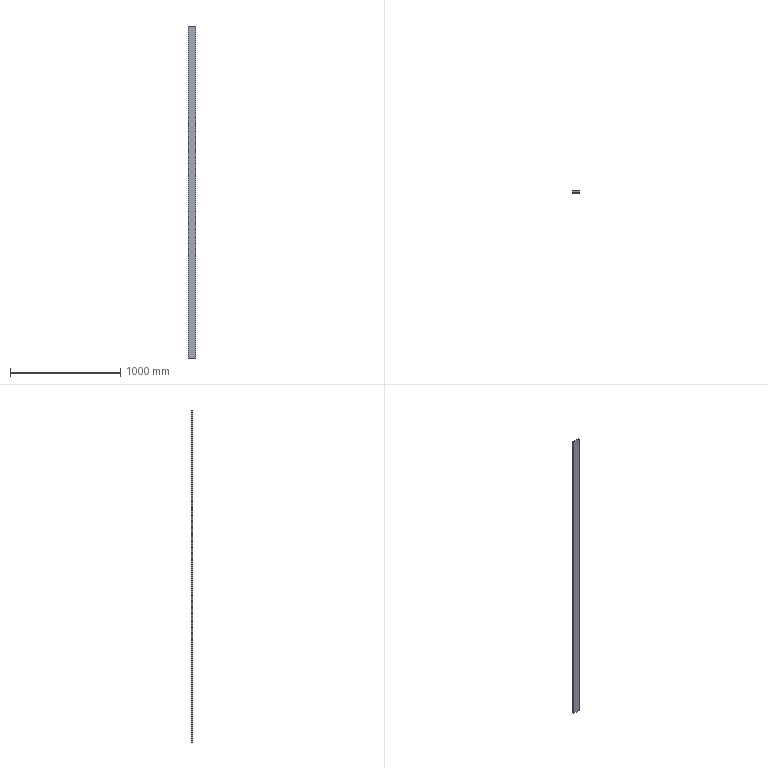Part | SolidWorks | features Extrusion 1 | 1 solid | 6 faces | box 70 x 14 x 3017 mm | volume 2956807 mm3 | plane 6
STEP:
#1=CARTESIAN_POINT('',(35.,-7.,0.));
#2=VERTEX_POINT('',#1);
#3=CARTESIAN_POINT('',(35.,7.,0.));
#4=VERTEX_POINT('',#3);
#5=CARTESIAN_POINT('',(35.,7.,0.));
#6=DIRECTION('',(0.,1.,0.));
#7=VECTOR('',#6,1000.);
#8=LINE('',#5,#7);
#9=EDGE_CURVE('',#2,#4,#8,.T.);
#10=ORIENTED_EDGE('',*,*,#9,.T.);
#11=CARTESIAN_POINT('',(35.,7.,3017.15));
#12=VERTEX_POINT('',#11);
#13=CARTESIAN_POINT('',(35.,7.,3017.15));
#14=DIRECTION('',(0.,0.,-1.));
#15=VECTOR('',#14,1000.);
#16=LINE('',#13,#15);
#17=EDGE_CURVE('',#12,#4,#16,.T.);
#18=ORIENTED_EDGE('',*,*,#17,.F.);
#19=CARTESIAN_POINT('',(35.,-7.,3017.15));
#20=VERTEX_POINT('',#19);
#21=CARTESIAN_POINT('',(35.,7.,3017.15));
#22=DIRECTION('',(0.,1.,0.));
#23=VECTOR('',#22,1000.);
#24=LINE('',#21,#23);
#25=EDGE_CURVE('',#20,#12,#24,.T.);
#26=ORIENTED_EDGE('',*,*,#25,.F.);
#27=CARTESIAN_POINT('',(35.,-7.,3017.15));
#28=DIRECTION('',(0.,0.,-1.));
#29=VECTOR('',#28,1000.);
#30=LINE('',#27,#29);
#31=EDGE_CURVE('',#20,#2,#30,.T.);
#32=ORIENTED_EDGE('',*,*,#31,.T.);
#33=EDGE_LOOP('',(#10,#18,#26,#32));
#34=FACE_OUTER_BOUND('',#33,.T.);
#35=CARTESIAN_POINT('',(35.,7.,3017.15));
#36=DIRECTION('',(-1.,0.,0.));
#37=DIRECTION('',(0.,0.,1.));
#38=AXIS2_PLACEMENT_3D('',#35,#36,#37);
#39=PLANE('',#38);
#40=ADVANCED_FACE('',(#34),#39,.F.);
#41=CARTESIAN_POINT('',(-35.,7.,0.));
#42=VERTEX_POINT('',#41);
#43=CARTESIAN_POINT('',(-35.,7.,0.));
#44=DIRECTION('',(-1.,0.,0.));
#45=VECTOR('',#44,1000.);
#46=LINE('',#43,#45);
#47=EDGE_CURVE('',#4,#42,#46,.T.);
#48=ORIENTED_EDGE('',*,*,#47,.T.);
#49=CARTESIAN_POINT('',(-35.,7.,3017.15));
#50=VERTEX_POINT('',#49);
#51=CARTESIAN_POINT('',(-35.,7.,3017.15));
#52=DIRECTION('',(0.,0.,-1.));
#53=VECTOR('',#52,1000.);
#54=LINE('',#51,#53);
#55=EDGE_CURVE('',#50,#42,#54,.T.);
#56=ORIENTED_EDGE('',*,*,#55,.F.);
#57=CARTESIAN_POINT('',(-35.,7.,3017.15));
#58=DIRECTION('',(-1.,0.,0.));
#59=VECTOR('',#58,1000.);
#60=LINE('',#57,#59);
#61=EDGE_CURVE('',#12,#50,#60,.T.);
#62=ORIENTED_EDGE('',*,*,#61,.F.);
#63=ORIENTED_EDGE('',*,*,#17,.T.);
#64=EDGE_LOOP('',(#48,#56,#62,#63));
#65=FACE_OUTER_BOUND('',#64,.T.);
#66=CARTESIAN_POINT('',(-35.,7.,3017.15));
#67=DIRECTION('',(0.,-1.,0.));
#68=DIRECTION('',(0.,0.,-1.));
#69=AXIS2_PLACEMENT_3D('',#66,#67,#68);
#70=PLANE('',#69);
#71=ADVANCED_FACE('',(#65),#70,.F.);
#72=CARTESIAN_POINT('',(-35.,-7.,0.));
#73=VERTEX_POINT('',#72);
#74=CARTESIAN_POINT('',(-35.,7.,0.));
#75=DIRECTION('',(0.,-1.,0.));
#76=VECTOR('',#75,1000.);
#77=LINE('',#74,#76);
#78=EDGE_CURVE('',#42,#73,#77,.T.);
#79=ORIENTED_EDGE('',*,*,#78,.T.);
#80=CARTESIAN_POINT('',(-35.,-7.,3017.15));
#81=VERTEX_POINT('',#80);
#82=CARTESIAN_POINT('',(-35.,-7.,3017.15));
#83=DIRECTION('',(0.,0.,-1.));
#84=VECTOR('',#83,1000.);
#85=LINE('',#82,#84);
#86=EDGE_CURVE('',#81,#73,#85,.T.);
#87=ORIENTED_EDGE('',*,*,#86,.F.);
#88=CARTESIAN_POINT('',(-35.,7.,3017.15));
#89=DIRECTION('',(0.,-1.,0.));
#90=VECTOR('',#89,1000.);
#91=LINE('',#88,#90);
#92=EDGE_CURVE('',#50,#81,#91,.T.);
#93=ORIENTED_EDGE('',*,*,#92,.F.);
#94=ORIENTED_EDGE('',*,*,#55,.T.);
#95=EDGE_LOOP('',(#79,#87,#93,#94));
#96=FACE_OUTER_BOUND('',#95,.T.);
#97=CARTESIAN_POINT('',(-35.,7.,3017.15));
#98=DIRECTION('',(1.,0.,0.));
#99=DIRECTION('',(0.,0.,-1.));
#100=AXIS2_PLACEMENT_3D('',#97,#98,#99);
#101=PLANE('',#100);
#102=ADVANCED_FACE('',(#96),#101,.F.);
#103=CARTESIAN_POINT('',(-35.,-7.,0.));
#104=DIRECTION('',(1.,0.,0.));
#105=VECTOR('',#104,1000.);
#106=LINE('',#103,#105);
#107=EDGE_CURVE('',#73,#2,#106,.T.);
#108=ORIENTED_EDGE('',*,*,#107,.T.);
#109=ORIENTED_EDGE('',*,*,#31,.F.);
#110=CARTESIAN_POINT('',(-35.,-7.,3017.15));
#111=DIRECTION('',(1.,0.,0.));
#112=VECTOR('',#111,1000.);
#113=LINE('',#110,#112);
#114=EDGE_CURVE('',#81,#20,#113,.T.);
#115=ORIENTED_EDGE('',*,*,#114,.F.);
#116=ORIENTED_EDGE('',*,*,#86,.T.);
#117=EDGE_LOOP('',(#108,#109,#115,#116));
#118=FACE_OUTER_BOUND('',#117,.T.);
#119=CARTESIAN_POINT('',(-35.,-7.,3017.15));
#120=DIRECTION('',(0.,1.,0.));
#121=DIRECTION('',(0.,0.,1.));
#122=AXIS2_PLACEMENT_3D('',#119,#120,#121);
#123=PLANE('',#122);
#124=ADVANCED_FACE('',(#118),#123,.F.);
#125=ORIENTED_EDGE('',*,*,#25,.T.);
#126=ORIENTED_EDGE('',*,*,#61,.T.);
#127=ORIENTED_EDGE('',*,*,#92,.T.);
#128=ORIENTED_EDGE('',*,*,#114,.T.);
#129=EDGE_LOOP('',(#125,#126,#127,#128));
#130=FACE_OUTER_BOUND('',#129,.T.);
#131=CARTESIAN_POINT('',(0.,0.,3017.15));
#132=DIRECTION('',(0.,0.,1.));
#133=DIRECTION('',(1.,0.,0.));
#134=AXIS2_PLACEMENT_3D('',#131,#132,#133);
#135=PLANE('',#134);
#136=ADVANCED_FACE('',(#130),#135,.T.);
#137=ORIENTED_EDGE('',*,*,#9,.F.);
#138=ORIENTED_EDGE('',*,*,#107,.F.);
#139=ORIENTED_EDGE('',*,*,#78,.F.);
#140=ORIENTED_EDGE('',*,*,#47,.F.);
#141=EDGE_LOOP('',(#137,#138,#139,#140));
#142=FACE_OUTER_BOUND('',#141,.T.);
#143=CARTESIAN_POINT('',(0.,0.,0.));
#144=DIRECTION('',(0.,0.,1.));
#145=DIRECTION('',(1.,0.,0.));
#146=AXIS2_PLACEMENT_3D('',#143,#144,#145);
#147=PLANE('',#146);
#148=ADVANCED_FACE('',(#142),#147,.F.);
#149=CLOSED_SHELL('',(#40,#71,#102,#124,#136,#148));
#150=MANIFOLD_SOLID_BREP('',#149);
#151=CARTESIAN_POINT('',(0.,0.,0.));
#152=DIRECTION('',(0.,0.,1.));
#153=DIRECTION('',(1.,0.,0.));
#154=AXIS2_PLACEMENT_3D('',#151,#152,#153);
#155=(LENGTH_UNIT()NAMED_UNIT(*)SI_UNIT(.MILLI.,.METRE.));
#156=UNCERTAINTY_MEASURE_WITH_UNIT(LENGTH_MEASURE(0.00001),#155,'','');
#157=(NAMED_UNIT(*)PLANE_ANGLE_UNIT()SI_UNIT($,.RADIAN.));
#158=(NAMED_UNIT(*)SI_UNIT($,.STERADIAN.)SOLID_ANGLE_UNIT());
#159=(GEOMETRIC_REPRESENTATION_CONTEXT(3)GLOBAL_UNCERTAINTY_ASSIGNED_CONTEXT((#156))GLOBAL_UNIT_ASSIGNED_CONTEXT((#155,#157,#158))REPRESENTATION_CONTEXT('',''));
#160=ADVANCED_BREP_SHAPE_REPRESENTATION('',(#150,#154),#159);